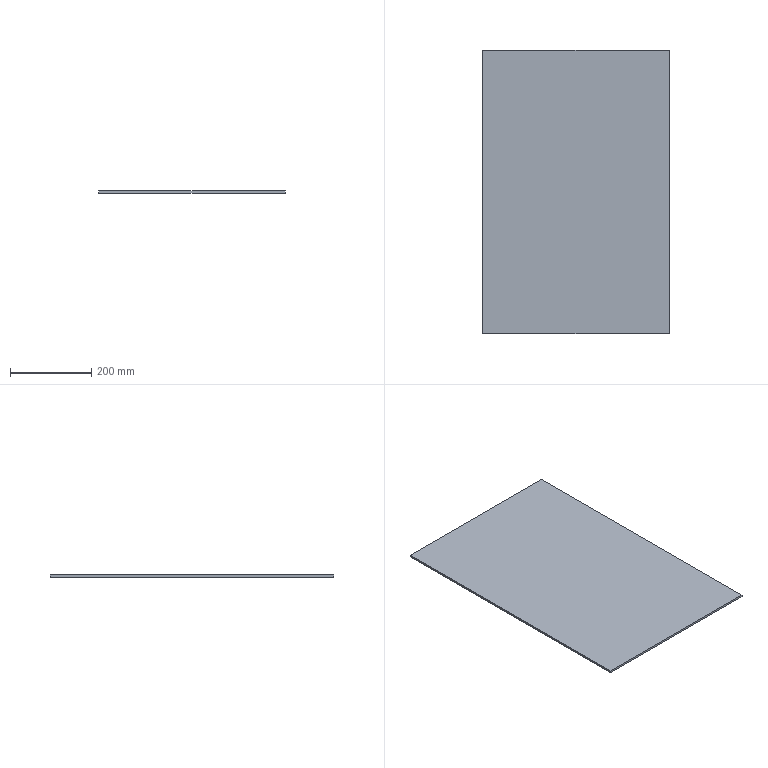Part | STEP file | 001-002-Panel | 1 solid | 6 faces | box 458 x 698 x 5 mm | volume 1598420 mm3 | plane 6
STEP:
#1=CARTESIAN_POINT('',(0.,0.,0.));
#2=DIRECTION('',(0.,0.,1.));
#3=DIRECTION('',(1.,0.,0.));
#4=AXIS2_PLACEMENT_3D('',#1,#2,#3);
#5=CARTESIAN_POINT('',(229.,-349.,0.));
#6=VERTEX_POINT('',#5);
#7=CARTESIAN_POINT('',(229.,349.,0.));
#8=VERTEX_POINT('',#7);
#9=CARTESIAN_POINT('',(229.,-349.,0.));
#10=DIRECTION('',(0.,1.,0.));
#11=VECTOR('',#10,1.);
#12=LINE('',#9,#11);
#13=CARTESIAN_POINT('',(229.,-349.,5.));
#14=DIRECTION('',(-1.,0.,0.));
#15=DIRECTION('',(0.,0.,1.));
#16=AXIS2_PLACEMENT_3D('',#13,#14,#15);
#17=PLANE('',#16);
#18=CARTESIAN_POINT('',(-5.,0.));
#19=DIRECTION('',(0.,1.));
#20=VECTOR('',#19,1.);
#21=LINE('',#18,#20);
#22=(GEOMETRIC_REPRESENTATION_CONTEXT(2)PARAMETRIC_REPRESENTATION_CONTEXT()REPRESENTATION_CONTEXT('',''));
#23=DEFINITIONAL_REPRESENTATION('',(#21),#22);
#24=PCURVE('',#17,#23);
#25=CARTESIAN_POINT('',(0.,0.,0.));
#26=DIRECTION('',(0.,0.,-1.));
#27=DIRECTION('',(-1.,0.,0.));
#28=AXIS2_PLACEMENT_3D('',#25,#26,#27);
#29=PLANE('',#28);
#30=CARTESIAN_POINT('',(-229.,-349.));
#31=DIRECTION('',(0.,1.));
#32=VECTOR('',#31,1.);
#33=LINE('',#30,#32);
#34=(GEOMETRIC_REPRESENTATION_CONTEXT(2)PARAMETRIC_REPRESENTATION_CONTEXT()REPRESENTATION_CONTEXT('',''));
#35=DEFINITIONAL_REPRESENTATION('',(#33),#34);
#36=PCURVE('',#29,#35);
#37=SURFACE_CURVE('',#12,(#24,#36),.PCURVE_S1.);
#38=EDGE_CURVE('',#6,#8,#37,.T.);
#39=ORIENTED_EDGE('',*,*,#38,.T.);
#40=CARTESIAN_POINT('',(229.,349.,5.));
#41=VERTEX_POINT('',#40);
#42=CARTESIAN_POINT('',(229.,349.,5.));
#43=DIRECTION('',(0.,0.,-1.));
#44=VECTOR('',#43,1.);
#45=LINE('',#42,#44);
#46=CARTESIAN_POINT('',(0.,698.));
#47=DIRECTION('',(-1.,0.));
#48=VECTOR('',#47,1.);
#49=LINE('',#46,#48);
#50=(GEOMETRIC_REPRESENTATION_CONTEXT(2)PARAMETRIC_REPRESENTATION_CONTEXT()REPRESENTATION_CONTEXT('',''));
#51=DEFINITIONAL_REPRESENTATION('',(#49),#50);
#52=PCURVE('',#17,#51);
#53=CARTESIAN_POINT('',(-229.,349.,5.));
#54=DIRECTION('',(0.,-1.,0.));
#55=DIRECTION('',(1.,0.,0.));
#56=AXIS2_PLACEMENT_3D('',#53,#54,#55);
#57=PLANE('',#56);
#58=CARTESIAN_POINT('',(458.,0.));
#59=DIRECTION('',(0.,-1.));
#60=VECTOR('',#59,1.);
#61=LINE('',#58,#60);
#62=(GEOMETRIC_REPRESENTATION_CONTEXT(2)PARAMETRIC_REPRESENTATION_CONTEXT()REPRESENTATION_CONTEXT('',''));
#63=DEFINITIONAL_REPRESENTATION('',(#61),#62);
#64=PCURVE('',#57,#63);
#65=SURFACE_CURVE('',#45,(#52,#64),.PCURVE_S1.);
#66=EDGE_CURVE('',#41,#8,#65,.T.);
#67=ORIENTED_EDGE('',*,*,#66,.F.);
#68=CARTESIAN_POINT('',(229.,-349.,5.));
#69=VERTEX_POINT('',#68);
#70=CARTESIAN_POINT('',(229.,-349.,5.));
#71=DIRECTION('',(0.,1.,0.));
#72=VECTOR('',#71,1.);
#73=LINE('',#70,#72);
#74=CARTESIAN_POINT('',(0.,0.));
#75=DIRECTION('',(0.,1.));
#76=VECTOR('',#75,1.);
#77=LINE('',#74,#76);
#78=(GEOMETRIC_REPRESENTATION_CONTEXT(2)PARAMETRIC_REPRESENTATION_CONTEXT()REPRESENTATION_CONTEXT('',''));
#79=DEFINITIONAL_REPRESENTATION('',(#77),#78);
#80=PCURVE('',#17,#79);
#81=CARTESIAN_POINT('',(0.,0.,5.));
#82=DIRECTION('',(0.,0.,-1.));
#83=DIRECTION('',(-1.,0.,0.));
#84=AXIS2_PLACEMENT_3D('',#81,#82,#83);
#85=PLANE('',#84);
#86=CARTESIAN_POINT('',(-229.,-349.));
#87=DIRECTION('',(0.,1.));
#88=VECTOR('',#87,1.);
#89=LINE('',#86,#88);
#90=(GEOMETRIC_REPRESENTATION_CONTEXT(2)PARAMETRIC_REPRESENTATION_CONTEXT()REPRESENTATION_CONTEXT('',''));
#91=DEFINITIONAL_REPRESENTATION('',(#89),#90);
#92=PCURVE('',#85,#91);
#93=SURFACE_CURVE('',#73,(#80,#92),.PCURVE_S1.);
#94=EDGE_CURVE('',#69,#41,#93,.T.);
#95=ORIENTED_EDGE('',*,*,#94,.F.);
#96=CARTESIAN_POINT('',(229.,-349.,5.));
#97=DIRECTION('',(0.,0.,-1.));
#98=VECTOR('',#97,1.);
#99=LINE('',#96,#98);
#100=CARTESIAN_POINT('',(0.,0.));
#101=DIRECTION('',(-1.,0.));
#102=VECTOR('',#101,1.);
#103=LINE('',#100,#102);
#104=(GEOMETRIC_REPRESENTATION_CONTEXT(2)PARAMETRIC_REPRESENTATION_CONTEXT()REPRESENTATION_CONTEXT('',''));
#105=DEFINITIONAL_REPRESENTATION('',(#103),#104);
#106=PCURVE('',#17,#105);
#107=CARTESIAN_POINT('',(-229.,-349.,5.));
#108=DIRECTION('',(0.,1.,0.));
#109=DIRECTION('',(0.,0.,1.));
#110=AXIS2_PLACEMENT_3D('',#107,#108,#109);
#111=PLANE('',#110);
#112=CARTESIAN_POINT('',(0.,458.));
#113=DIRECTION('',(-1.,0.));
#114=VECTOR('',#113,1.);
#115=LINE('',#112,#114);
#116=(GEOMETRIC_REPRESENTATION_CONTEXT(2)PARAMETRIC_REPRESENTATION_CONTEXT()REPRESENTATION_CONTEXT('',''));
#117=DEFINITIONAL_REPRESENTATION('',(#115),#116);
#118=PCURVE('',#111,#117);
#119=SURFACE_CURVE('',#99,(#106,#118),.PCURVE_S1.);
#120=EDGE_CURVE('',#69,#6,#119,.T.);
#121=ORIENTED_EDGE('',*,*,#120,.T.);
#122=EDGE_LOOP('',(#39,#67,#95,#121));
#123=FACE_BOUND('',#122,.T.);
#124=ADVANCED_FACE('',(#123),#17,.F.);
#125=CARTESIAN_POINT('',(-229.,349.,0.));
#126=VERTEX_POINT('',#125);
#127=CARTESIAN_POINT('',(-229.,349.,0.));
#128=DIRECTION('',(-1.,0.,0.));
#129=VECTOR('',#128,1.);
#130=LINE('',#127,#129);
#131=CARTESIAN_POINT('',(0.,-5.));
#132=DIRECTION('',(-1.,0.));
#133=VECTOR('',#132,1.);
#134=LINE('',#131,#133);
#135=(GEOMETRIC_REPRESENTATION_CONTEXT(2)PARAMETRIC_REPRESENTATION_CONTEXT()REPRESENTATION_CONTEXT('',''));
#136=DEFINITIONAL_REPRESENTATION('',(#134),#135);
#137=PCURVE('',#57,#136);
#138=CARTESIAN_POINT('',(229.,349.));
#139=DIRECTION('',(1.,0.));
#140=VECTOR('',#139,1.);
#141=LINE('',#138,#140);
#142=(GEOMETRIC_REPRESENTATION_CONTEXT(2)PARAMETRIC_REPRESENTATION_CONTEXT()REPRESENTATION_CONTEXT('',''));
#143=DEFINITIONAL_REPRESENTATION('',(#141),#142);
#144=PCURVE('',#29,#143);
#145=SURFACE_CURVE('',#130,(#137,#144),.PCURVE_S1.);
#146=EDGE_CURVE('',#8,#126,#145,.T.);
#147=ORIENTED_EDGE('',*,*,#146,.T.);
#148=CARTESIAN_POINT('',(-229.,349.,5.));
#149=VERTEX_POINT('',#148);
#150=CARTESIAN_POINT('',(-229.,349.,5.));
#151=DIRECTION('',(0.,0.,-1.));
#152=VECTOR('',#151,1.);
#153=LINE('',#150,#152);
#154=CARTESIAN_POINT('',(0.,0.));
#155=DIRECTION('',(0.,-1.));
#156=VECTOR('',#155,1.);
#157=LINE('',#154,#156);
#158=(GEOMETRIC_REPRESENTATION_CONTEXT(2)PARAMETRIC_REPRESENTATION_CONTEXT()REPRESENTATION_CONTEXT('',''));
#159=DEFINITIONAL_REPRESENTATION('',(#157),#158);
#160=PCURVE('',#57,#159);
#161=CARTESIAN_POINT('',(-229.,-349.,5.));
#162=DIRECTION('',(1.,0.,0.));
#163=DIRECTION('',(0.,0.,-1.));
#164=AXIS2_PLACEMENT_3D('',#161,#162,#163);
#165=PLANE('',#164);
#166=CARTESIAN_POINT('',(0.,698.));
#167=DIRECTION('',(1.,0.));
#168=VECTOR('',#167,1.);
#169=LINE('',#166,#168);
#170=(GEOMETRIC_REPRESENTATION_CONTEXT(2)PARAMETRIC_REPRESENTATION_CONTEXT()REPRESENTATION_CONTEXT('',''));
#171=DEFINITIONAL_REPRESENTATION('',(#169),#170);
#172=PCURVE('',#165,#171);
#173=SURFACE_CURVE('',#153,(#160,#172),.PCURVE_S1.);
#174=EDGE_CURVE('',#149,#126,#173,.T.);
#175=ORIENTED_EDGE('',*,*,#174,.F.);
#176=CARTESIAN_POINT('',(-229.,349.,5.));
#177=DIRECTION('',(-1.,0.,0.));
#178=VECTOR('',#177,1.);
#179=LINE('',#176,#178);
#180=CARTESIAN_POINT('',(0.,0.));
#181=DIRECTION('',(-1.,0.));
#182=VECTOR('',#181,1.);
#183=LINE('',#180,#182);
#184=(GEOMETRIC_REPRESENTATION_CONTEXT(2)PARAMETRIC_REPRESENTATION_CONTEXT()REPRESENTATION_CONTEXT('',''));
#185=DEFINITIONAL_REPRESENTATION('',(#183),#184);
#186=PCURVE('',#57,#185);
#187=CARTESIAN_POINT('',(229.,349.));
#188=DIRECTION('',(1.,0.));
#189=VECTOR('',#188,1.);
#190=LINE('',#187,#189);
#191=(GEOMETRIC_REPRESENTATION_CONTEXT(2)PARAMETRIC_REPRESENTATION_CONTEXT()REPRESENTATION_CONTEXT('',''));
#192=DEFINITIONAL_REPRESENTATION('',(#190),#191);
#193=PCURVE('',#85,#192);
#194=SURFACE_CURVE('',#179,(#186,#193),.PCURVE_S1.);
#195=EDGE_CURVE('',#41,#149,#194,.T.);
#196=ORIENTED_EDGE('',*,*,#195,.F.);
#197=ORIENTED_EDGE('',*,*,#66,.T.);
#198=EDGE_LOOP('',(#147,#175,#196,#197));
#199=FACE_BOUND('',#198,.T.);
#200=ADVANCED_FACE('',(#199),#57,.F.);
#201=CARTESIAN_POINT('',(-229.,-349.,0.));
#202=VERTEX_POINT('',#201);
#203=CARTESIAN_POINT('',(-229.,-349.,0.));
#204=DIRECTION('',(0.,-1.,0.));
#205=VECTOR('',#204,1.);
#206=LINE('',#203,#205);
#207=CARTESIAN_POINT('',(5.,0.));
#208=DIRECTION('',(0.,-1.));
#209=VECTOR('',#208,1.);
#210=LINE('',#207,#209);
#211=(GEOMETRIC_REPRESENTATION_CONTEXT(2)PARAMETRIC_REPRESENTATION_CONTEXT()REPRESENTATION_CONTEXT('',''));
#212=DEFINITIONAL_REPRESENTATION('',(#210),#211);
#213=PCURVE('',#165,#212);
#214=CARTESIAN_POINT('',(229.,-349.));
#215=DIRECTION('',(0.,-1.));
#216=VECTOR('',#215,1.);
#217=LINE('',#214,#216);
#218=(GEOMETRIC_REPRESENTATION_CONTEXT(2)PARAMETRIC_REPRESENTATION_CONTEXT()REPRESENTATION_CONTEXT('',''));
#219=DEFINITIONAL_REPRESENTATION('',(#217),#218);
#220=PCURVE('',#29,#219);
#221=SURFACE_CURVE('',#206,(#213,#220),.PCURVE_S1.);
#222=EDGE_CURVE('',#126,#202,#221,.T.);
#223=ORIENTED_EDGE('',*,*,#222,.T.);
#224=CARTESIAN_POINT('',(-229.,-349.,5.));
#225=VERTEX_POINT('',#224);
#226=CARTESIAN_POINT('',(-229.,-349.,5.));
#227=DIRECTION('',(0.,0.,-1.));
#228=VECTOR('',#227,1.);
#229=LINE('',#226,#228);
#230=CARTESIAN_POINT('',(0.,0.));
#231=DIRECTION('',(1.,0.));
#232=VECTOR('',#231,1.);
#233=LINE('',#230,#232);
#234=(GEOMETRIC_REPRESENTATION_CONTEXT(2)PARAMETRIC_REPRESENTATION_CONTEXT()REPRESENTATION_CONTEXT('',''));
#235=DEFINITIONAL_REPRESENTATION('',(#233),#234);
#236=PCURVE('',#165,#235);
#237=CARTESIAN_POINT('',(0.,0.));
#238=DIRECTION('',(-1.,0.));
#239=VECTOR('',#238,1.);
#240=LINE('',#237,#239);
#241=(GEOMETRIC_REPRESENTATION_CONTEXT(2)PARAMETRIC_REPRESENTATION_CONTEXT()REPRESENTATION_CONTEXT('',''));
#242=DEFINITIONAL_REPRESENTATION('',(#240),#241);
#243=PCURVE('',#111,#242);
#244=SURFACE_CURVE('',#229,(#236,#243),.PCURVE_S1.);
#245=EDGE_CURVE('',#225,#202,#244,.T.);
#246=ORIENTED_EDGE('',*,*,#245,.F.);
#247=CARTESIAN_POINT('',(-229.,-349.,5.));
#248=DIRECTION('',(0.,-1.,0.));
#249=VECTOR('',#248,1.);
#250=LINE('',#247,#249);
#251=CARTESIAN_POINT('',(0.,0.));
#252=DIRECTION('',(0.,-1.));
#253=VECTOR('',#252,1.);
#254=LINE('',#251,#253);
#255=(GEOMETRIC_REPRESENTATION_CONTEXT(2)PARAMETRIC_REPRESENTATION_CONTEXT()REPRESENTATION_CONTEXT('',''));
#256=DEFINITIONAL_REPRESENTATION('',(#254),#255);
#257=PCURVE('',#165,#256);
#258=CARTESIAN_POINT('',(229.,-349.));
#259=DIRECTION('',(0.,-1.));
#260=VECTOR('',#259,1.);
#261=LINE('',#258,#260);
#262=(GEOMETRIC_REPRESENTATION_CONTEXT(2)PARAMETRIC_REPRESENTATION_CONTEXT()REPRESENTATION_CONTEXT('',''));
#263=DEFINITIONAL_REPRESENTATION('',(#261),#262);
#264=PCURVE('',#85,#263);
#265=SURFACE_CURVE('',#250,(#257,#264),.PCURVE_S1.);
#266=EDGE_CURVE('',#149,#225,#265,.T.);
#267=ORIENTED_EDGE('',*,*,#266,.F.);
#268=ORIENTED_EDGE('',*,*,#174,.T.);
#269=EDGE_LOOP('',(#223,#246,#267,#268));
#270=FACE_BOUND('',#269,.T.);
#271=ADVANCED_FACE('',(#270),#165,.F.);
#272=CARTESIAN_POINT('',(-229.,-349.,0.));
#273=DIRECTION('',(1.,0.,0.));
#274=VECTOR('',#273,1.);
#275=LINE('',#272,#274);
#276=CARTESIAN_POINT('',(-5.,0.));
#277=DIRECTION('',(0.,1.));
#278=VECTOR('',#277,1.);
#279=LINE('',#276,#278);
#280=(GEOMETRIC_REPRESENTATION_CONTEXT(2)PARAMETRIC_REPRESENTATION_CONTEXT()REPRESENTATION_CONTEXT('',''));
#281=DEFINITIONAL_REPRESENTATION('',(#279),#280);
#282=PCURVE('',#111,#281);
#283=CARTESIAN_POINT('',(229.,-349.));
#284=DIRECTION('',(-1.,0.));
#285=VECTOR('',#284,1.);
#286=LINE('',#283,#285);
#287=(GEOMETRIC_REPRESENTATION_CONTEXT(2)PARAMETRIC_REPRESENTATION_CONTEXT()REPRESENTATION_CONTEXT('',''));
#288=DEFINITIONAL_REPRESENTATION('',(#286),#287);
#289=PCURVE('',#29,#288);
#290=SURFACE_CURVE('',#275,(#282,#289),.PCURVE_S1.);
#291=EDGE_CURVE('',#202,#6,#290,.T.);
#292=ORIENTED_EDGE('',*,*,#291,.T.);
#293=ORIENTED_EDGE('',*,*,#120,.F.);
#294=CARTESIAN_POINT('',(-229.,-349.,5.));
#295=DIRECTION('',(1.,0.,0.));
#296=VECTOR('',#295,1.);
#297=LINE('',#294,#296);
#298=CARTESIAN_POINT('',(0.,0.));
#299=DIRECTION('',(0.,1.));
#300=VECTOR('',#299,1.);
#301=LINE('',#298,#300);
#302=(GEOMETRIC_REPRESENTATION_CONTEXT(2)PARAMETRIC_REPRESENTATION_CONTEXT()REPRESENTATION_CONTEXT('',''));
#303=DEFINITIONAL_REPRESENTATION('',(#301),#302);
#304=PCURVE('',#111,#303);
#305=CARTESIAN_POINT('',(229.,-349.));
#306=DIRECTION('',(-1.,0.));
#307=VECTOR('',#306,1.);
#308=LINE('',#305,#307);
#309=(GEOMETRIC_REPRESENTATION_CONTEXT(2)PARAMETRIC_REPRESENTATION_CONTEXT()REPRESENTATION_CONTEXT('',''));
#310=DEFINITIONAL_REPRESENTATION('',(#308),#309);
#311=PCURVE('',#85,#310);
#312=SURFACE_CURVE('',#297,(#304,#311),.PCURVE_S1.);
#313=EDGE_CURVE('',#225,#69,#312,.T.);
#314=ORIENTED_EDGE('',*,*,#313,.F.);
#315=ORIENTED_EDGE('',*,*,#245,.T.);
#316=EDGE_LOOP('',(#292,#293,#314,#315));
#317=FACE_BOUND('',#316,.T.);
#318=ADVANCED_FACE('',(#317),#111,.F.);
#319=ORIENTED_EDGE('',*,*,#94,.T.);
#320=ORIENTED_EDGE('',*,*,#195,.T.);
#321=ORIENTED_EDGE('',*,*,#266,.T.);
#322=ORIENTED_EDGE('',*,*,#313,.T.);
#323=EDGE_LOOP('',(#319,#320,#321,#322));
#324=FACE_BOUND('',#323,.T.);
#325=ADVANCED_FACE('',(#324),#85,.F.);
#326=ORIENTED_EDGE('',*,*,#38,.F.);
#327=ORIENTED_EDGE('',*,*,#291,.F.);
#328=ORIENTED_EDGE('',*,*,#222,.F.);
#329=ORIENTED_EDGE('',*,*,#146,.F.);
#330=EDGE_LOOP('',(#326,#327,#328,#329));
#331=FACE_BOUND('',#330,.T.);
#332=ADVANCED_FACE('',(#331),#29,.T.);
#333=CLOSED_SHELL('',(#124,#200,#271,#318,#325,#332));
#334=MANIFOLD_SOLID_BREP('',#333);
#335=(LENGTH_UNIT()NAMED_UNIT(*)SI_UNIT(.MILLI.,.METRE.));
#336=UNCERTAINTY_MEASURE_WITH_UNIT(LENGTH_MEASURE(0.0000001),#335,'','');
#337=(NAMED_UNIT(*)PLANE_ANGLE_UNIT()SI_UNIT($,.RADIAN.));
#338=(NAMED_UNIT(*)SI_UNIT($,.STERADIAN.)SOLID_ANGLE_UNIT());
#339=(GEOMETRIC_REPRESENTATION_CONTEXT(3)GLOBAL_UNCERTAINTY_ASSIGNED_CONTEXT((#336))GLOBAL_UNIT_ASSIGNED_CONTEXT((#335,#337,#338))REPRESENTATION_CONTEXT('',''));
#340=ADVANCED_BREP_SHAPE_REPRESENTATION('',(#4,#334),#339);